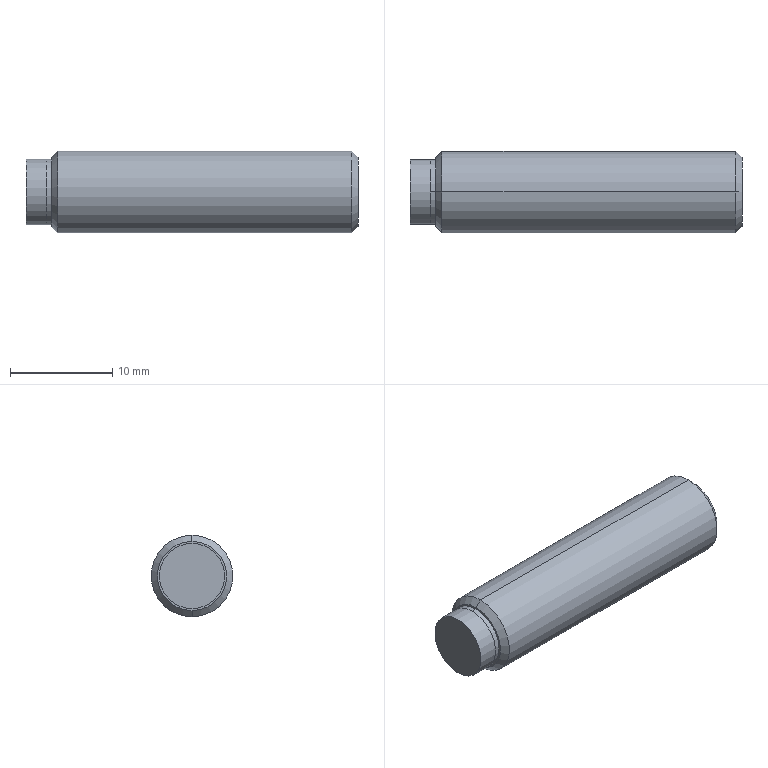Part | NX | features BREP 2 | 2 solids | 14 faces | box 32.5 x 8 x 8 mm | volume 1579 mm3 | plane 5 | cylinder 5 | cone 4 | commonest cylinder face diameters 6.4 x3 8 x2
STEP:
#1=CARTESIAN_POINT('',(0.,0.,3.2));
#2=VERTEX_POINT('',#1);
#3=CARTESIAN_POINT('',(0.,0.,-3.2));
#4=VERTEX_POINT('',#3);
#5=CARTESIAN_POINT('',(0.,0.,0.));
#6=DIRECTION('',(1.,0.,0.));
#7=DIRECTION('',(0.,0.,-1.));
#8=AXIS2_PLACEMENT_3D('',#5,#6,#7);
#9=CIRCLE('',#8,3.2);
#10=EDGE_CURVE('',#2,#4,#9,.T.);
#11=ORIENTED_EDGE('',*,*,#10,.F.);
#12=CARTESIAN_POINT('',(0.,0.,0.));
#13=DIRECTION('',(1.,0.,0.));
#14=DIRECTION('',(0.,0.,-1.));
#15=AXIS2_PLACEMENT_3D('',#12,#13,#14);
#16=CIRCLE('',#15,3.2);
#17=EDGE_CURVE('',#4,#2,#16,.T.);
#18=ORIENTED_EDGE('',*,*,#17,.F.);
#19=EDGE_LOOP('',(#11,#18));
#20=FACE_BOUND('',#19,.T.);
#21=CARTESIAN_POINT('',(0.,0.,0.));
#22=DIRECTION('',(1.,0.,0.));
#23=DIRECTION('',(0.,0.,1.));
#24=AXIS2_PLACEMENT_3D('',#21,#22,#23);
#25=PLANE('',#24);
#26=ADVANCED_FACE('',(#20),#25,.F.);
#27=CARTESIAN_POINT('',(0.5,0.,3.2));
#28=VERTEX_POINT('',#27);
#29=CARTESIAN_POINT('',(0.,0.,3.2));
#30=DIRECTION('',(1.,0.,0.));
#31=VECTOR('',#30,1000.);
#32=LINE('',#29,#31);
#33=EDGE_CURVE('',#28,#2,#32,.F.);
#34=ORIENTED_EDGE('',*,*,#33,.F.);
#35=CARTESIAN_POINT('',(0.5,0.,-3.2));
#36=VERTEX_POINT('',#35);
#37=CARTESIAN_POINT('',(0.5,0.,0.));
#38=DIRECTION('',(1.,0.,0.));
#39=DIRECTION('',(0.,0.,-1.));
#40=AXIS2_PLACEMENT_3D('',#37,#38,#39);
#41=CIRCLE('',#40,3.2);
#42=EDGE_CURVE('',#36,#28,#41,.T.);
#43=ORIENTED_EDGE('',*,*,#42,.F.);
#44=CARTESIAN_POINT('',(0.,0.,-3.2));
#45=DIRECTION('',(1.,0.,0.));
#46=VECTOR('',#45,1000.);
#47=LINE('',#44,#46);
#48=EDGE_CURVE('',#36,#4,#47,.F.);
#49=ORIENTED_EDGE('',*,*,#48,.T.);
#50=ORIENTED_EDGE('',*,*,#17,.T.);
#51=EDGE_LOOP('',(#34,#43,#49,#50));
#52=FACE_BOUND('',#51,.T.);
#53=CARTESIAN_POINT('',(0.5,0.,0.));
#54=DIRECTION('',(1.,0.,0.));
#55=DIRECTION('',(0.,1.,0.));
#56=AXIS2_PLACEMENT_3D('',#53,#54,#55);
#57=CYLINDRICAL_SURFACE('',#56,3.2);
#58=ADVANCED_FACE('',(#52),#57,.T.);
#59=ORIENTED_EDGE('',*,*,#33,.T.);
#60=ORIENTED_EDGE('',*,*,#10,.T.);
#61=ORIENTED_EDGE('',*,*,#48,.F.);
#62=CARTESIAN_POINT('',(0.5,0.,0.));
#63=DIRECTION('',(1.,0.,0.));
#64=DIRECTION('',(0.,0.,-1.));
#65=AXIS2_PLACEMENT_3D('',#62,#63,#64);
#66=CIRCLE('',#65,3.2);
#67=EDGE_CURVE('',#28,#36,#66,.T.);
#68=ORIENTED_EDGE('',*,*,#67,.F.);
#69=EDGE_LOOP('',(#59,#60,#61,#68));
#70=FACE_BOUND('',#69,.T.);
#71=CARTESIAN_POINT('',(0.5,0.,0.));
#72=DIRECTION('',(1.,0.,0.));
#73=DIRECTION('',(0.,-1.,0.));
#74=AXIS2_PLACEMENT_3D('',#71,#72,#73);
#75=CYLINDRICAL_SURFACE('',#74,3.2);
#76=ADVANCED_FACE('',(#70),#75,.T.);
#77=CARTESIAN_POINT('',(0.5,0.,3.386));
#78=VERTEX_POINT('',#77);
#79=CARTESIAN_POINT('',(0.5,0.,-3.386));
#80=VERTEX_POINT('',#79);
#81=CARTESIAN_POINT('',(0.5,0.,0.));
#82=DIRECTION('',(1.,0.,0.));
#83=DIRECTION('',(0.,0.,-1.));
#84=AXIS2_PLACEMENT_3D('',#81,#82,#83);
#85=CIRCLE('',#84,3.386);
#86=EDGE_CURVE('',#78,#80,#85,.T.);
#87=ORIENTED_EDGE('',*,*,#86,.F.);
#88=CARTESIAN_POINT('',(0.5,0.,0.));
#89=DIRECTION('',(1.,0.,0.));
#90=DIRECTION('',(0.,0.,-1.));
#91=AXIS2_PLACEMENT_3D('',#88,#89,#90);
#92=CIRCLE('',#91,3.386);
#93=EDGE_CURVE('',#80,#78,#92,.T.);
#94=ORIENTED_EDGE('',*,*,#93,.F.);
#95=EDGE_LOOP('',(#87,#94));
#96=FACE_BOUND('',#95,.T.);
#97=ORIENTED_EDGE('',*,*,#42,.T.);
#98=ORIENTED_EDGE('',*,*,#67,.T.);
#99=EDGE_LOOP('',(#97,#98));
#100=FACE_BOUND('',#99,.T.);
#101=CARTESIAN_POINT('',(0.5,0.,0.));
#102=DIRECTION('',(1.,0.,0.));
#103=DIRECTION('',(0.,0.,1.));
#104=AXIS2_PLACEMENT_3D('',#101,#102,#103);
#105=PLANE('',#104);
#106=ADVANCED_FACE('',(#96,#100),#105,.F.);
#107=CARTESIAN_POINT('',(1.113,0.,4.));
#108=VERTEX_POINT('',#107);
#109=CARTESIAN_POINT('',(0.5,0.,3.386));
#110=DIRECTION('',(0.7071,0.,0.7071));
#111=VECTOR('',#110,1000.);
#112=LINE('',#109,#111);
#113=EDGE_CURVE('',#108,#78,#112,.F.);
#114=ORIENTED_EDGE('',*,*,#113,.F.);
#115=CARTESIAN_POINT('',(1.113,0.,-4.));
#116=VERTEX_POINT('',#115);
#117=CARTESIAN_POINT('',(1.113,0.,0.));
#118=DIRECTION('',(1.,0.,0.));
#119=DIRECTION('',(0.,0.,-1.));
#120=AXIS2_PLACEMENT_3D('',#117,#118,#119);
#121=CIRCLE('',#120,4.);
#122=EDGE_CURVE('',#116,#108,#121,.T.);
#123=ORIENTED_EDGE('',*,*,#122,.F.);
#124=CARTESIAN_POINT('',(0.5,0.,-3.386));
#125=DIRECTION('',(0.7071,0.,-0.7071));
#126=VECTOR('',#125,1000.);
#127=LINE('',#124,#126);
#128=EDGE_CURVE('',#116,#80,#127,.F.);
#129=ORIENTED_EDGE('',*,*,#128,.T.);
#130=ORIENTED_EDGE('',*,*,#93,.T.);
#131=EDGE_LOOP('',(#114,#123,#129,#130));
#132=FACE_BOUND('',#131,.T.);
#133=CARTESIAN_POINT('',(0.5,0.,0.));
#134=DIRECTION('',(1.,0.,0.));
#135=DIRECTION('',(0.,1.,0.));
#136=AXIS2_PLACEMENT_3D('',#133,#134,#135);
#137=CONICAL_SURFACE('',#136,3.386,0.7854);
#138=ADVANCED_FACE('',(#132),#137,.T.);
#139=ORIENTED_EDGE('',*,*,#113,.T.);
#140=ORIENTED_EDGE('',*,*,#86,.T.);
#141=ORIENTED_EDGE('',*,*,#128,.F.);
#142=CARTESIAN_POINT('',(1.113,0.,0.));
#143=DIRECTION('',(1.,0.,0.));
#144=DIRECTION('',(0.,0.,-1.));
#145=AXIS2_PLACEMENT_3D('',#142,#143,#144);
#146=CIRCLE('',#145,4.);
#147=EDGE_CURVE('',#108,#116,#146,.T.);
#148=ORIENTED_EDGE('',*,*,#147,.F.);
#149=EDGE_LOOP('',(#139,#140,#141,#148));
#150=FACE_BOUND('',#149,.T.);
#151=CARTESIAN_POINT('',(0.5,0.,0.));
#152=DIRECTION('',(1.,0.,0.));
#153=DIRECTION('',(0.,-1.,0.));
#154=AXIS2_PLACEMENT_3D('',#151,#152,#153);
#155=CONICAL_SURFACE('',#154,3.386,0.7854);
#156=ADVANCED_FACE('',(#150),#155,.T.);
#157=CARTESIAN_POINT('',(29.887,0.,4.));
#158=VERTEX_POINT('',#157);
#159=CARTESIAN_POINT('',(1.113,0.,4.));
#160=DIRECTION('',(1.,0.,0.));
#161=VECTOR('',#160,1000.);
#162=LINE('',#159,#161);
#163=EDGE_CURVE('',#108,#158,#162,.T.);
#164=ORIENTED_EDGE('',*,*,#163,.F.);
#165=ORIENTED_EDGE('',*,*,#147,.T.);
#166=CARTESIAN_POINT('',(29.887,0.,-4.));
#167=VERTEX_POINT('',#166);
#168=CARTESIAN_POINT('',(1.113,0.,-4.));
#169=DIRECTION('',(1.,0.,0.));
#170=VECTOR('',#169,1000.);
#171=LINE('',#168,#170);
#172=EDGE_CURVE('',#116,#167,#171,.T.);
#173=ORIENTED_EDGE('',*,*,#172,.T.);
#174=CARTESIAN_POINT('',(29.887,0.,0.));
#175=DIRECTION('',(1.,0.,0.));
#176=DIRECTION('',(0.,0.,-1.));
#177=AXIS2_PLACEMENT_3D('',#174,#175,#176);
#178=CIRCLE('',#177,4.);
#179=EDGE_CURVE('',#158,#167,#178,.T.);
#180=ORIENTED_EDGE('',*,*,#179,.F.);
#181=EDGE_LOOP('',(#164,#165,#173,#180));
#182=FACE_BOUND('',#181,.T.);
#183=CARTESIAN_POINT('',(30.5,0.,0.));
#184=DIRECTION('',(1.,0.,0.));
#185=DIRECTION('',(0.,-1.,0.000000001));
#186=AXIS2_PLACEMENT_3D('',#183,#184,#185);
#187=CYLINDRICAL_SURFACE('',#186,4.);
#188=ADVANCED_FACE('',(#182),#187,.T.);
#189=CARTESIAN_POINT('',(30.5,0.,-3.386));
#190=VERTEX_POINT('',#189);
#191=CARTESIAN_POINT('',(30.5,0.,-3.386));
#192=DIRECTION('',(-0.7071,0.,-0.7071));
#193=VECTOR('',#192,1000.);
#194=LINE('',#191,#193);
#195=EDGE_CURVE('',#167,#190,#194,.F.);
#196=ORIENTED_EDGE('',*,*,#195,.T.);
#197=CARTESIAN_POINT('',(30.5,0.,3.386));
#198=VERTEX_POINT('',#197);
#199=CARTESIAN_POINT('',(30.5,0.,0.));
#200=DIRECTION('',(1.,0.,0.));
#201=DIRECTION('',(0.,0.,-1.));
#202=AXIS2_PLACEMENT_3D('',#199,#200,#201);
#203=CIRCLE('',#202,3.386);
#204=EDGE_CURVE('',#198,#190,#203,.T.);
#205=ORIENTED_EDGE('',*,*,#204,.F.);
#206=CARTESIAN_POINT('',(30.5,0.,3.386));
#207=DIRECTION('',(-0.7071,0.,0.7071));
#208=VECTOR('',#207,1000.);
#209=LINE('',#206,#208);
#210=EDGE_CURVE('',#158,#198,#209,.F.);
#211=ORIENTED_EDGE('',*,*,#210,.F.);
#212=ORIENTED_EDGE('',*,*,#179,.T.);
#213=EDGE_LOOP('',(#196,#205,#211,#212));
#214=FACE_BOUND('',#213,.T.);
#215=CARTESIAN_POINT('',(29.887,0.,0.));
#216=DIRECTION('',(-1.,0.,0.));
#217=DIRECTION('',(0.,-1.,0.));
#218=AXIS2_PLACEMENT_3D('',#215,#216,#217);
#219=CONICAL_SURFACE('',#218,4.,0.7854);
#220=ADVANCED_FACE('',(#214),#219,.T.);
#221=ORIENTED_EDGE('',*,*,#195,.F.);
#222=CARTESIAN_POINT('',(29.887,0.,0.));
#223=DIRECTION('',(1.,0.,0.));
#224=DIRECTION('',(0.,0.,-1.));
#225=AXIS2_PLACEMENT_3D('',#222,#223,#224);
#226=CIRCLE('',#225,4.);
#227=EDGE_CURVE('',#167,#158,#226,.T.);
#228=ORIENTED_EDGE('',*,*,#227,.T.);
#229=ORIENTED_EDGE('',*,*,#210,.T.);
#230=CARTESIAN_POINT('',(30.5,0.,0.));
#231=DIRECTION('',(1.,0.,0.));
#232=DIRECTION('',(0.,0.,-1.));
#233=AXIS2_PLACEMENT_3D('',#230,#231,#232);
#234=CIRCLE('',#233,3.386);
#235=EDGE_CURVE('',#190,#198,#234,.T.);
#236=ORIENTED_EDGE('',*,*,#235,.F.);
#237=EDGE_LOOP('',(#221,#228,#229,#236));
#238=FACE_BOUND('',#237,.T.);
#239=CARTESIAN_POINT('',(29.887,0.,0.));
#240=DIRECTION('',(-1.,0.,0.));
#241=DIRECTION('',(0.,1.,0.));
#242=AXIS2_PLACEMENT_3D('',#239,#240,#241);
#243=CONICAL_SURFACE('',#242,4.,0.7854);
#244=ADVANCED_FACE('',(#238),#243,.T.);
#245=ORIENTED_EDGE('',*,*,#235,.T.);
#246=ORIENTED_EDGE('',*,*,#204,.T.);
#247=EDGE_LOOP('',(#245,#246));
#248=FACE_BOUND('',#247,.T.);
#249=CARTESIAN_POINT('',(30.5,3.386,0.));
#250=DIRECTION('',(-1.,0.,0.));
#251=DIRECTION('',(0.,0.,-1.));
#252=AXIS2_PLACEMENT_3D('',#249,#250,#251);
#253=PLANE('',#252);
#254=ADVANCED_FACE('',(#248),#253,.F.);
#255=ORIENTED_EDGE('',*,*,#163,.T.);
#256=ORIENTED_EDGE('',*,*,#227,.F.);
#257=ORIENTED_EDGE('',*,*,#172,.F.);
#258=ORIENTED_EDGE('',*,*,#122,.T.);
#259=EDGE_LOOP('',(#255,#256,#257,#258));
#260=FACE_BOUND('',#259,.T.);
#261=CARTESIAN_POINT('',(30.5,0.,0.));
#262=DIRECTION('',(1.,0.,0.));
#263=DIRECTION('',(0.,1.,0.000000001));
#264=AXIS2_PLACEMENT_3D('',#261,#262,#263);
#265=CYLINDRICAL_SURFACE('',#264,4.);
#266=ADVANCED_FACE('',(#260),#265,.T.);
#267=CLOSED_SHELL('',(#26,#58,#76,#106,#138,#156,#188,#220,#244,#254,#266));
#268=MANIFOLD_SOLID_BREP('',#267);
#269=CARTESIAN_POINT('',(-2.,0.,3.2));
#270=VERTEX_POINT('',#269);
#271=CARTESIAN_POINT('',(-2.,0.,0.));
#272=DIRECTION('',(-1.,0.,0.));
#273=DIRECTION('',(0.,0.,1.));
#274=AXIS2_PLACEMENT_3D('',#271,#272,#273);
#275=CIRCLE('',#274,3.2);
#276=EDGE_CURVE('',#270,#270,#275,.T.);
#277=ORIENTED_EDGE('',*,*,#276,.F.);
#278=EDGE_LOOP('',(#277));
#279=FACE_BOUND('',#278,.T.);
#280=CARTESIAN_POINT('',(0.,0.,3.2));
#281=VERTEX_POINT('',#280);
#282=CARTESIAN_POINT('',(0.,0.,0.));
#283=DIRECTION('',(-1.,0.,0.));
#284=DIRECTION('',(0.,0.,1.));
#285=AXIS2_PLACEMENT_3D('',#282,#283,#284);
#286=CIRCLE('',#285,3.2);
#287=EDGE_CURVE('',#281,#281,#286,.T.);
#288=ORIENTED_EDGE('',*,*,#287,.T.);
#289=EDGE_LOOP('',(#288));
#290=FACE_BOUND('',#289,.T.);
#291=CARTESIAN_POINT('',(-2.,0.,0.));
#292=DIRECTION('',(1.,0.,0.));
#293=DIRECTION('',(0.,0.,1.));
#294=AXIS2_PLACEMENT_3D('',#291,#292,#293);
#295=CYLINDRICAL_SURFACE('',#294,3.2);
#296=ADVANCED_FACE('',(#279,#290),#295,.T.);
#297=ORIENTED_EDGE('',*,*,#276,.T.);
#298=EDGE_LOOP('',(#297));
#299=FACE_BOUND('',#298,.T.);
#300=CARTESIAN_POINT('',(-2.,0.,0.));
#301=DIRECTION('',(-1.,0.,0.));
#302=DIRECTION('',(0.,0.,-1.));
#303=AXIS2_PLACEMENT_3D('',#300,#301,#302);
#304=PLANE('',#303);
#305=ADVANCED_FACE('',(#299),#304,.T.);
#306=ORIENTED_EDGE('',*,*,#287,.F.);
#307=EDGE_LOOP('',(#306));
#308=FACE_BOUND('',#307,.T.);
#309=CARTESIAN_POINT('',(0.,0.,0.));
#310=DIRECTION('',(-1.,0.,0.));
#311=DIRECTION('',(0.,0.,-1.));
#312=AXIS2_PLACEMENT_3D('',#309,#310,#311);
#313=PLANE('',#312);
#314=ADVANCED_FACE('',(#308),#313,.F.);
#315=CLOSED_SHELL('',(#296,#305,#314));
#316=MANIFOLD_SOLID_BREP('',#315);
#317=(LENGTH_UNIT()NAMED_UNIT(*)SI_UNIT(.MILLI.,.METRE.));
#318=UNCERTAINTY_MEASURE_WITH_UNIT(LENGTH_MEASURE(0.00001),#317,'','');
#319=(NAMED_UNIT(*)PLANE_ANGLE_UNIT()SI_UNIT($,.RADIAN.));
#320=(NAMED_UNIT(*)SI_UNIT($,.STERADIAN.)SOLID_ANGLE_UNIT());
#321=(GEOMETRIC_REPRESENTATION_CONTEXT(3)GLOBAL_UNCERTAINTY_ASSIGNED_CONTEXT((#318))GLOBAL_UNIT_ASSIGNED_CONTEXT((#317,#319,#320))REPRESENTATION_CONTEXT('',''));
#322=ADVANCED_BREP_SHAPE_REPRESENTATION('',(#268,#316),#321);